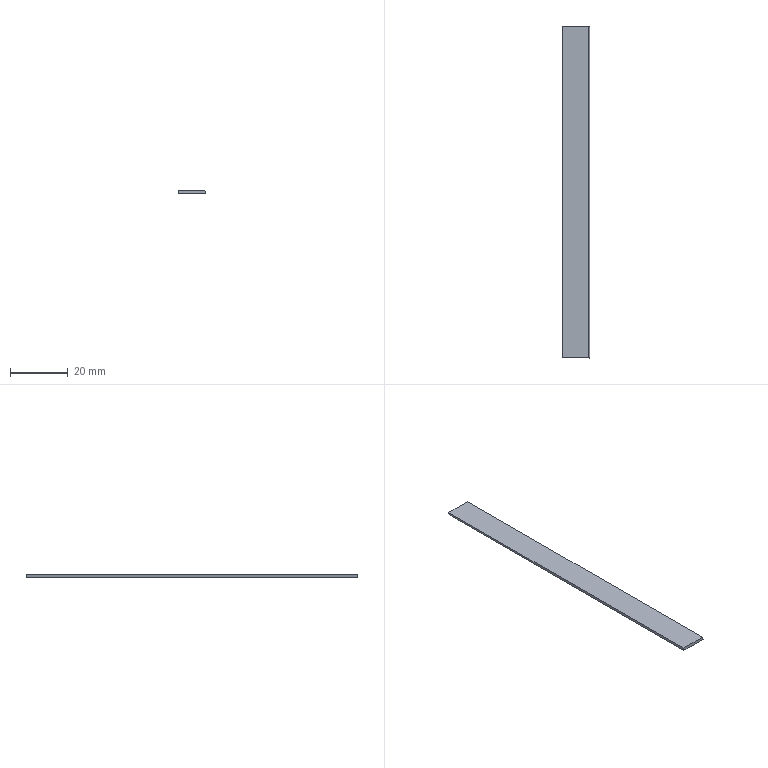Part | SolidWorks | features BaseBody 1 | 1 solid | 6 faces | box 9.702 x 115.104 x 1.056 mm | volume 1139 mm3 | plane 4 | cylinder 2 | commonest cylinder face diameters 97.2 x1 165.792 x1
STEP:
#1=CARTESIAN_POINT('',(-2177.883,1269.344,-1596.144));
#2=VERTEX_POINT('',#1);
#3=CARTESIAN_POINT('',(-2177.883,1154.24,-1596.144));
#4=VERTEX_POINT('',#3);
#5=CARTESIAN_POINT('',(-2177.883,1269.344,-1596.144));
#6=DIRECTION('',(0.,-1.,0.));
#7=VECTOR('',#6,1000.);
#8=LINE('',#5,#7);
#9=EDGE_CURVE('',#2,#4,#8,.T.);
#10=ORIENTED_EDGE('',*,*,#9,.F.);
#11=CARTESIAN_POINT('',(-2178.304,1269.344,-1595.088));
#12=VERTEX_POINT('',#11);
#13=CARTESIAN_POINT('',(-2132.95,1269.344,-1577.624));
#14=DIRECTION('',(0.,1.,0.));
#15=DIRECTION('',(-0.9246,0.,-0.3811));
#16=AXIS2_PLACEMENT_3D('',#13,#14,#15);
#17=CIRCLE('',#16,48.6);
#18=EDGE_CURVE('',#2,#12,#17,.T.);
#19=ORIENTED_EDGE('',*,*,#18,.T.);
#20=CARTESIAN_POINT('',(-2178.304,1154.24,-1595.088));
#21=VERTEX_POINT('',#20);
#22=CARTESIAN_POINT('',(-2178.304,1269.344,-1595.088));
#23=DIRECTION('',(0.,-1.,0.));
#24=VECTOR('',#23,1000.);
#25=LINE('',#22,#24);
#26=EDGE_CURVE('',#12,#21,#25,.T.);
#27=ORIENTED_EDGE('',*,*,#26,.T.);
#28=CARTESIAN_POINT('',(-2132.95,1154.24,-1577.624));
#29=DIRECTION('',(0.,-1.,0.));
#30=DIRECTION('',(-0.9332,0.,-0.3593));
#31=AXIS2_PLACEMENT_3D('',#28,#29,#30);
#32=CIRCLE('',#31,48.6);
#33=EDGE_CURVE('',#21,#4,#32,.T.);
#34=ORIENTED_EDGE('',*,*,#33,.T.);
#35=EDGE_LOOP('',(#10,#19,#27,#34));
#36=FACE_OUTER_BOUND('',#35,.T.);
#37=CARTESIAN_POINT('',(-2132.95,1275.099,-1577.624));
#38=DIRECTION('',(0.,-1.,0.));
#39=DIRECTION('',(-0.961,0.,-0.2766));
#40=AXIS2_PLACEMENT_3D('',#37,#38,#39);
#41=CYLINDRICAL_SURFACE('',#40,48.6);
#42=ADVANCED_FACE('',(#36),#41,.F.);
#43=CARTESIAN_POINT('',(-2187.351,1269.344,-1596.144));
#44=VERTEX_POINT('',#43);
#45=CARTESIAN_POINT('',(-2187.351,1154.24,-1596.144));
#46=VERTEX_POINT('',#45);
#47=CARTESIAN_POINT('',(-2187.351,1269.344,-1596.144));
#48=DIRECTION('',(0.,-1.,0.));
#49=VECTOR('',#48,1000.);
#50=LINE('',#47,#49);
#51=EDGE_CURVE('',#44,#46,#50,.T.);
#52=ORIENTED_EDGE('',*,*,#51,.T.);
#53=CARTESIAN_POINT('',(-2187.585,1154.24,-1595.088));
#54=VERTEX_POINT('',#53);
#55=CARTESIAN_POINT('',(-2106.55,1154.24,-1577.624));
#56=DIRECTION('',(0.,-1.,0.));
#57=DIRECTION('',(-0.9776,0.,-0.2107));
#58=AXIS2_PLACEMENT_3D('',#55,#56,#57);
#59=CIRCLE('',#58,82.896);
#60=EDGE_CURVE('',#54,#46,#59,.T.);
#61=ORIENTED_EDGE('',*,*,#60,.F.);
#62=CARTESIAN_POINT('',(-2187.585,1269.344,-1595.088));
#63=VERTEX_POINT('',#62);
#64=CARTESIAN_POINT('',(-2187.585,1154.24,-1595.088));
#65=DIRECTION('',(0.,1.,0.));
#66=VECTOR('',#65,1000.);
#67=LINE('',#64,#66);
#68=EDGE_CURVE('',#54,#63,#67,.T.);
#69=ORIENTED_EDGE('',*,*,#68,.T.);
#70=CARTESIAN_POINT('',(-2106.55,1269.344,-1577.624));
#71=DIRECTION('',(0.,1.,0.));
#72=DIRECTION('',(-0.9747,0.,-0.2234));
#73=AXIS2_PLACEMENT_3D('',#70,#71,#72);
#74=CIRCLE('',#73,82.896);
#75=EDGE_CURVE('',#44,#63,#74,.T.);
#76=ORIENTED_EDGE('',*,*,#75,.F.);
#77=EDGE_LOOP('',(#52,#61,#69,#76));
#78=FACE_OUTER_BOUND('',#77,.T.);
#79=CARTESIAN_POINT('',(-2106.55,1275.099,-1577.624));
#80=DIRECTION('',(0.,1.,0.));
#81=DIRECTION('',(-0.9515,0.,-0.3075));
#82=AXIS2_PLACEMENT_3D('',#79,#80,#81);
#83=CYLINDRICAL_SURFACE('',#82,82.896);
#84=ADVANCED_FACE('',(#78),#83,.T.);
#85=ORIENTED_EDGE('',*,*,#68,.F.);
#86=CARTESIAN_POINT('',(-2178.304,1154.24,-1595.088));
#87=DIRECTION('',(-1.,0.,0.));
#88=VECTOR('',#87,1000.);
#89=LINE('',#86,#88);
#90=EDGE_CURVE('',#21,#54,#89,.T.);
#91=ORIENTED_EDGE('',*,*,#90,.F.);
#92=ORIENTED_EDGE('',*,*,#26,.F.);
#93=CARTESIAN_POINT('',(-2187.585,1269.344,-1595.088));
#94=DIRECTION('',(1.,0.,0.));
#95=VECTOR('',#94,1000.);
#96=LINE('',#93,#95);
#97=EDGE_CURVE('',#63,#12,#96,.T.);
#98=ORIENTED_EDGE('',*,*,#97,.F.);
#99=EDGE_LOOP('',(#85,#91,#92,#98));
#100=FACE_OUTER_BOUND('',#99,.T.);
#101=CARTESIAN_POINT('',(-2172.549,1275.099,-1595.088));
#102=DIRECTION('',(0.,0.,1.));
#103=DIRECTION('',(1.,0.,0.));
#104=AXIS2_PLACEMENT_3D('',#101,#102,#103);
#105=PLANE('',#104);
#106=ADVANCED_FACE('',(#100),#105,.T.);
#107=ORIENTED_EDGE('',*,*,#18,.F.);
#108=CARTESIAN_POINT('',(-2177.883,1269.344,-1596.144));
#109=DIRECTION('',(-1.,-0.000000003,0.));
#110=VECTOR('',#109,1000.);
#111=LINE('',#108,#110);
#112=EDGE_CURVE('',#2,#44,#111,.T.);
#113=ORIENTED_EDGE('',*,*,#112,.T.);
#114=ORIENTED_EDGE('',*,*,#75,.T.);
#115=ORIENTED_EDGE('',*,*,#97,.T.);
#116=EDGE_LOOP('',(#107,#113,#114,#115));
#117=FACE_OUTER_BOUND('',#116,.T.);
#118=CARTESIAN_POINT('',(-2188.071,1269.344,-1596.629));
#119=DIRECTION('',(0.,1.,0.));
#120=DIRECTION('',(1.,0.,0.));
#121=AXIS2_PLACEMENT_3D('',#118,#119,#120);
#122=PLANE('',#121);
#123=ADVANCED_FACE('',(#117),#122,.T.);
#124=ORIENTED_EDGE('',*,*,#33,.F.);
#125=ORIENTED_EDGE('',*,*,#90,.T.);
#126=ORIENTED_EDGE('',*,*,#60,.T.);
#127=CARTESIAN_POINT('',(-2187.351,1154.24,-1596.144));
#128=DIRECTION('',(1.,-0.000000003,0.));
#129=VECTOR('',#128,1000.);
#130=LINE('',#127,#129);
#131=EDGE_CURVE('',#46,#4,#130,.T.);
#132=ORIENTED_EDGE('',*,*,#131,.T.);
#133=EDGE_LOOP('',(#124,#125,#126,#132));
#134=FACE_OUTER_BOUND('',#133,.T.);
#135=CARTESIAN_POINT('',(-2177.398,1154.24,-1594.602));
#136=DIRECTION('',(0.,-1.,0.));
#137=DIRECTION('',(0.,0.,-1.));
#138=AXIS2_PLACEMENT_3D('',#135,#136,#137);
#139=PLANE('',#138);
#140=ADVANCED_FACE('',(#134),#139,.T.);
#141=ORIENTED_EDGE('',*,*,#9,.T.);
#142=ORIENTED_EDGE('',*,*,#131,.F.);
#143=ORIENTED_EDGE('',*,*,#51,.F.);
#144=ORIENTED_EDGE('',*,*,#112,.F.);
#145=EDGE_LOOP('',(#141,#142,#143,#144));
#146=FACE_OUTER_BOUND('',#145,.T.);
#147=CARTESIAN_POINT('',(-2193.106,1275.099,-1596.144));
#148=DIRECTION('',(0.,0.,-1.));
#149=DIRECTION('',(0.,-1.,0.));
#150=AXIS2_PLACEMENT_3D('',#147,#148,#149);
#151=PLANE('',#150);
#152=ADVANCED_FACE('',(#146),#151,.T.);
#153=CLOSED_SHELL('',(#42,#84,#106,#123,#140,#152));
#154=MANIFOLD_SOLID_BREP('',#153);
#155=CARTESIAN_POINT('',(0.,0.,0.));
#156=DIRECTION('',(0.,0.,1.));
#157=DIRECTION('',(1.,0.,0.));
#158=AXIS2_PLACEMENT_3D('',#155,#156,#157);
#159=(LENGTH_UNIT()NAMED_UNIT(*)SI_UNIT(.MILLI.,.METRE.));
#160=UNCERTAINTY_MEASURE_WITH_UNIT(LENGTH_MEASURE(0.00001),#159,'','');
#161=(NAMED_UNIT(*)PLANE_ANGLE_UNIT()SI_UNIT($,.RADIAN.));
#162=(NAMED_UNIT(*)SI_UNIT($,.STERADIAN.)SOLID_ANGLE_UNIT());
#163=(GEOMETRIC_REPRESENTATION_CONTEXT(3)GLOBAL_UNCERTAINTY_ASSIGNED_CONTEXT((#160))GLOBAL_UNIT_ASSIGNED_CONTEXT((#159,#161,#162))REPRESENTATION_CONTEXT('',''));
#164=ADVANCED_BREP_SHAPE_REPRESENTATION('',(#154,#158),#163);